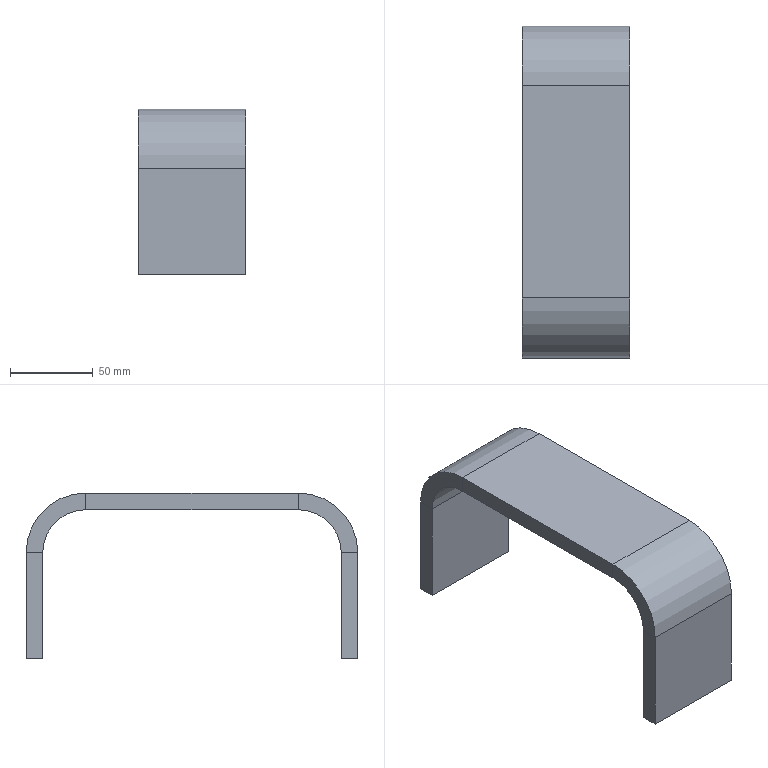Part | SolidWorks | features FlatPattern 1, SM3dBend 1, SMBaseFlange 1, SheetMetal 1 | 1 solid | 22 faces | box 65 x 200.003 x 99.994 mm | volume 229697 mm3 | plane 18 | cylinder 4 | commonest cylinder face diameters 52 x2 72 x2
STEP:
#1=CARTESIAN_POINT('',(904.458,674.984,0.));
#2=VERTEX_POINT('',#1);
#3=CARTESIAN_POINT('',(904.458,802.987,0.));
#4=VERTEX_POINT('',#3);
#5=CARTESIAN_POINT('',(904.458,562.296,0.));
#6=DIRECTION('',(0.,1.,0.));
#7=VECTOR('',#6,1000.);
#8=LINE('',#5,#7);
#9=EDGE_CURVE('',#2,#4,#8,.T.);
#10=ORIENTED_EDGE('',*,*,#9,.T.);
#11=CARTESIAN_POINT('',(839.458,802.987,0.));
#12=VERTEX_POINT('',#11);
#13=CARTESIAN_POINT('',(0.,802.987,0.));
#14=DIRECTION('',(-1.,0.,0.));
#15=VECTOR('',#14,1000.);
#16=LINE('',#13,#15);
#17=EDGE_CURVE('',#4,#12,#16,.T.);
#18=ORIENTED_EDGE('',*,*,#17,.T.);
#19=CARTESIAN_POINT('',(839.458,674.984,0.));
#20=VERTEX_POINT('',#19);
#21=CARTESIAN_POINT('',(839.458,915.676,0.));
#22=DIRECTION('',(0.,-1.,0.));
#23=VECTOR('',#22,1000.);
#24=LINE('',#21,#23);
#25=EDGE_CURVE('',#12,#20,#24,.T.);
#26=ORIENTED_EDGE('',*,*,#25,.T.);
#27=CARTESIAN_POINT('',(0.,674.984,0.));
#28=DIRECTION('',(-1.,0.,0.));
#29=VECTOR('',#28,1000.);
#30=LINE('',#27,#29);
#31=EDGE_CURVE('',#2,#20,#30,.T.);
#32=ORIENTED_EDGE('',*,*,#31,.F.);
#33=EDGE_LOOP('',(#10,#18,#26,#32));
#34=FACE_OUTER_BOUND('',#33,.T.);
#35=CARTESIAN_POINT('',(0.,0.,0.));
#36=DIRECTION('',(0.,0.,-1.));
#37=DIRECTION('',(-1.,0.,0.));
#38=AXIS2_PLACEMENT_3D('',#35,#36,#37);
#39=PLANE('',#38);
#40=ADVANCED_FACE('',(#34),#39,.F.);
#41=CARTESIAN_POINT('',(904.458,802.987,-10.));
#42=VERTEX_POINT('',#41);
#43=CARTESIAN_POINT('',(904.458,802.987,-10.));
#44=DIRECTION('',(0.,0.,-1.));
#45=VECTOR('',#44,1000.);
#46=LINE('',#43,#45);
#47=EDGE_CURVE('',#4,#42,#46,.T.);
#48=ORIENTED_EDGE('',*,*,#47,.F.);
#49=ORIENTED_EDGE('',*,*,#9,.F.);
#50=CARTESIAN_POINT('',(904.458,674.984,-10.));
#51=VERTEX_POINT('',#50);
#52=CARTESIAN_POINT('',(904.458,674.984,-10.));
#53=DIRECTION('',(0.,0.,-1.));
#54=VECTOR('',#53,1000.);
#55=LINE('',#52,#54);
#56=EDGE_CURVE('',#2,#51,#55,.T.);
#57=ORIENTED_EDGE('',*,*,#56,.T.);
#58=CARTESIAN_POINT('',(904.458,562.296,-10.));
#59=DIRECTION('',(0.,1.,0.));
#60=VECTOR('',#59,1000.);
#61=LINE('',#58,#60);
#62=EDGE_CURVE('',#51,#42,#61,.T.);
#63=ORIENTED_EDGE('',*,*,#62,.T.);
#64=EDGE_LOOP('',(#48,#49,#57,#63));
#65=FACE_OUTER_BOUND('',#64,.T.);
#66=CARTESIAN_POINT('',(904.458,562.296,-10.));
#67=DIRECTION('',(1.,0.,0.));
#68=DIRECTION('',(0.,0.,-1.));
#69=AXIS2_PLACEMENT_3D('',#66,#67,#68);
#70=PLANE('',#69);
#71=ADVANCED_FACE('',(#65),#70,.T.);
#72=CARTESIAN_POINT('',(839.458,802.987,-10.));
#73=VERTEX_POINT('',#72);
#74=CARTESIAN_POINT('',(839.458,802.987,-10.));
#75=DIRECTION('',(0.,0.,1.));
#76=VECTOR('',#75,1000.);
#77=LINE('',#74,#76);
#78=EDGE_CURVE('',#73,#12,#77,.T.);
#79=ORIENTED_EDGE('',*,*,#78,.F.);
#80=CARTESIAN_POINT('',(839.458,674.984,-10.));
#81=VERTEX_POINT('',#80);
#82=CARTESIAN_POINT('',(839.458,915.676,-10.));
#83=DIRECTION('',(0.,-1.,0.));
#84=VECTOR('',#83,1000.);
#85=LINE('',#82,#84);
#86=EDGE_CURVE('',#73,#81,#85,.T.);
#87=ORIENTED_EDGE('',*,*,#86,.T.);
#88=CARTESIAN_POINT('',(839.458,674.984,-10.));
#89=DIRECTION('',(0.,0.,1.));
#90=VECTOR('',#89,1000.);
#91=LINE('',#88,#90);
#92=EDGE_CURVE('',#81,#20,#91,.T.);
#93=ORIENTED_EDGE('',*,*,#92,.T.);
#94=ORIENTED_EDGE('',*,*,#25,.F.);
#95=EDGE_LOOP('',(#79,#87,#93,#94));
#96=FACE_OUTER_BOUND('',#95,.T.);
#97=CARTESIAN_POINT('',(839.458,915.676,-10.));
#98=DIRECTION('',(-1.,0.,0.));
#99=DIRECTION('',(0.,0.,1.));
#100=AXIS2_PLACEMENT_3D('',#97,#98,#99);
#101=PLANE('',#100);
#102=ADVANCED_FACE('',(#96),#101,.T.);
#103=CARTESIAN_POINT('',(0.,802.987,-10.));
#104=DIRECTION('',(-1.,0.,0.));
#105=VECTOR('',#104,1000.);
#106=LINE('',#103,#105);
#107=EDGE_CURVE('',#42,#73,#106,.T.);
#108=ORIENTED_EDGE('',*,*,#107,.F.);
#109=ORIENTED_EDGE('',*,*,#62,.F.);
#110=CARTESIAN_POINT('',(0.,674.984,-10.));
#111=DIRECTION('',(-1.,0.,0.));
#112=VECTOR('',#111,1000.);
#113=LINE('',#110,#112);
#114=EDGE_CURVE('',#51,#81,#113,.T.);
#115=ORIENTED_EDGE('',*,*,#114,.T.);
#116=ORIENTED_EDGE('',*,*,#86,.F.);
#117=EDGE_LOOP('',(#108,#109,#115,#116));
#118=FACE_OUTER_BOUND('',#117,.T.);
#119=CARTESIAN_POINT('',(0.,0.,-10.));
#120=DIRECTION('',(0.,0.,-1.));
#121=DIRECTION('',(-1.,0.,0.));
#122=AXIS2_PLACEMENT_3D('',#119,#120,#121);
#123=PLANE('',#122);
#124=ADVANCED_FACE('',(#118),#123,.T.);
#125=ORIENTED_EDGE('',*,*,#56,.F.);
#126=CARTESIAN_POINT('',(904.458,638.984,-36.));
#127=VERTEX_POINT('',#126);
#128=CARTESIAN_POINT('',(904.458,674.984,-36.));
#129=DIRECTION('',(1.,0.,0.));
#130=DIRECTION('',(0.,0.,1.));
#131=AXIS2_PLACEMENT_3D('',#128,#129,#130);
#132=CIRCLE('',#131,36.);
#133=EDGE_CURVE('',#2,#127,#132,.T.);
#134=ORIENTED_EDGE('',*,*,#133,.T.);
#135=CARTESIAN_POINT('',(904.458,648.984,-36.));
#136=VERTEX_POINT('',#135);
#137=CARTESIAN_POINT('',(904.458,648.984,-36.));
#138=DIRECTION('',(0.,1.,0.));
#139=VECTOR('',#138,1000.);
#140=LINE('',#137,#139);
#141=EDGE_CURVE('',#127,#136,#140,.T.);
#142=ORIENTED_EDGE('',*,*,#141,.T.);
#143=CARTESIAN_POINT('',(904.458,674.984,-36.));
#144=DIRECTION('',(1.,0.,0.));
#145=DIRECTION('',(0.,0.,1.));
#146=AXIS2_PLACEMENT_3D('',#143,#144,#145);
#147=CIRCLE('',#146,26.);
#148=EDGE_CURVE('',#51,#136,#147,.T.);
#149=ORIENTED_EDGE('',*,*,#148,.F.);
#150=EDGE_LOOP('',(#125,#134,#142,#149));
#151=FACE_OUTER_BOUND('',#150,.T.);
#152=CARTESIAN_POINT('',(904.458,674.984,-36.));
#153=DIRECTION('',(-1.,0.,0.));
#154=DIRECTION('',(0.,0.,1.));
#155=AXIS2_PLACEMENT_3D('',#152,#153,#154);
#156=PLANE('',#155);
#157=ADVANCED_FACE('',(#151),#156,.F.);
#158=CARTESIAN_POINT('',(839.458,638.984,-36.));
#159=VERTEX_POINT('',#158);
#160=CARTESIAN_POINT('',(839.458,674.984,-36.));
#161=DIRECTION('',(-1.,0.,0.));
#162=DIRECTION('',(0.,0.,1.));
#163=AXIS2_PLACEMENT_3D('',#160,#161,#162);
#164=CIRCLE('',#163,36.);
#165=EDGE_CURVE('',#159,#20,#164,.T.);
#166=ORIENTED_EDGE('',*,*,#165,.T.);
#167=ORIENTED_EDGE('',*,*,#92,.F.);
#168=CARTESIAN_POINT('',(839.458,648.984,-36.));
#169=VERTEX_POINT('',#168);
#170=CARTESIAN_POINT('',(839.458,674.984,-36.));
#171=DIRECTION('',(-1.,0.,0.));
#172=DIRECTION('',(0.,0.,-1.));
#173=AXIS2_PLACEMENT_3D('',#170,#171,#172);
#174=CIRCLE('',#173,26.);
#175=EDGE_CURVE('',#169,#81,#174,.T.);
#176=ORIENTED_EDGE('',*,*,#175,.F.);
#177=CARTESIAN_POINT('',(839.458,648.984,-36.));
#178=DIRECTION('',(0.,-1.,0.));
#179=VECTOR('',#178,1000.);
#180=LINE('',#177,#179);
#181=EDGE_CURVE('',#169,#159,#180,.T.);
#182=ORIENTED_EDGE('',*,*,#181,.T.);
#183=EDGE_LOOP('',(#166,#167,#176,#182));
#184=FACE_OUTER_BOUND('',#183,.T.);
#185=CARTESIAN_POINT('',(839.458,674.984,-36.));
#186=DIRECTION('',(1.,0.,0.));
#187=DIRECTION('',(0.,0.,-1.));
#188=AXIS2_PLACEMENT_3D('',#185,#186,#187);
#189=PLANE('',#188);
#190=ADVANCED_FACE('',(#184),#189,.F.);
#191=CARTESIAN_POINT('',(0.,648.984,-36.));
#192=DIRECTION('',(-1.,0.,0.));
#193=VECTOR('',#192,1000.);
#194=LINE('',#191,#193);
#195=EDGE_CURVE('',#136,#169,#194,.T.);
#196=ORIENTED_EDGE('',*,*,#195,.T.);
#197=ORIENTED_EDGE('',*,*,#175,.T.);
#198=ORIENTED_EDGE('',*,*,#114,.F.);
#199=ORIENTED_EDGE('',*,*,#148,.T.);
#200=EDGE_LOOP('',(#196,#197,#198,#199));
#201=FACE_OUTER_BOUND('',#200,.T.);
#202=CARTESIAN_POINT('',(953.788,674.984,-36.));
#203=DIRECTION('',(-1.,0.,0.));
#204=DIRECTION('',(0.,0.,1.));
#205=AXIS2_PLACEMENT_3D('',#202,#203,#204);
#206=CYLINDRICAL_SURFACE('',#205,26.);
#207=ADVANCED_FACE('',(#201),#206,.F.);
#208=CARTESIAN_POINT('',(0.,638.984,-36.));
#209=DIRECTION('',(-1.,0.,0.));
#210=VECTOR('',#209,1000.);
#211=LINE('',#208,#210);
#212=EDGE_CURVE('',#127,#159,#211,.T.);
#213=ORIENTED_EDGE('',*,*,#212,.F.);
#214=ORIENTED_EDGE('',*,*,#133,.F.);
#215=ORIENTED_EDGE('',*,*,#31,.T.);
#216=ORIENTED_EDGE('',*,*,#165,.F.);
#217=EDGE_LOOP('',(#213,#214,#215,#216));
#218=FACE_OUTER_BOUND('',#217,.T.);
#219=CARTESIAN_POINT('',(953.788,674.984,-36.));
#220=DIRECTION('',(-1.,0.,0.));
#221=DIRECTION('',(0.,0.,1.));
#222=AXIS2_PLACEMENT_3D('',#219,#220,#221);
#223=CYLINDRICAL_SURFACE('',#222,36.);
#224=ADVANCED_FACE('',(#218),#223,.T.);
#225=CARTESIAN_POINT('',(839.458,638.984,-99.994));
#226=VERTEX_POINT('',#225);
#227=CARTESIAN_POINT('',(904.458,638.984,-99.994));
#228=VERTEX_POINT('',#227);
#229=CARTESIAN_POINT('',(839.458,638.984,-99.994));
#230=DIRECTION('',(1.,0.,0.));
#231=VECTOR('',#230,1000.);
#232=LINE('',#229,#231);
#233=EDGE_CURVE('',#226,#228,#232,.T.);
#234=ORIENTED_EDGE('',*,*,#233,.F.);
#235=CARTESIAN_POINT('',(839.458,648.984,-99.994));
#236=VERTEX_POINT('',#235);
#237=CARTESIAN_POINT('',(839.458,648.984,-99.994));
#238=DIRECTION('',(0.,-1.,0.));
#239=VECTOR('',#238,1000.);
#240=LINE('',#237,#239);
#241=EDGE_CURVE('',#236,#226,#240,.T.);
#242=ORIENTED_EDGE('',*,*,#241,.F.);
#243=CARTESIAN_POINT('',(904.458,648.984,-99.994));
#244=VERTEX_POINT('',#243);
#245=CARTESIAN_POINT('',(839.458,648.984,-99.994));
#246=DIRECTION('',(1.,0.,0.));
#247=VECTOR('',#246,1000.);
#248=LINE('',#245,#247);
#249=EDGE_CURVE('',#236,#244,#248,.T.);
#250=ORIENTED_EDGE('',*,*,#249,.T.);
#251=CARTESIAN_POINT('',(904.458,648.984,-99.994));
#252=DIRECTION('',(0.,-1.,0.));
#253=VECTOR('',#252,1000.);
#254=LINE('',#251,#253);
#255=EDGE_CURVE('',#244,#228,#254,.T.);
#256=ORIENTED_EDGE('',*,*,#255,.T.);
#257=EDGE_LOOP('',(#234,#242,#250,#256));
#258=FACE_OUTER_BOUND('',#257,.T.);
#259=CARTESIAN_POINT('',(839.458,648.984,-99.994));
#260=DIRECTION('',(0.,0.,-1.));
#261=DIRECTION('',(1.,0.,0.));
#262=AXIS2_PLACEMENT_3D('',#259,#260,#261);
#263=PLANE('',#262);
#264=ADVANCED_FACE('',(#258),#263,.T.);
#265=ORIENTED_EDGE('',*,*,#195,.F.);
#266=CARTESIAN_POINT('',(904.458,648.984,-99.994));
#267=DIRECTION('',(0.,0.,1.));
#268=VECTOR('',#267,1000.);
#269=LINE('',#266,#268);
#270=EDGE_CURVE('',#244,#136,#269,.T.);
#271=ORIENTED_EDGE('',*,*,#270,.F.);
#272=ORIENTED_EDGE('',*,*,#249,.F.);
#273=CARTESIAN_POINT('',(839.458,648.984,253.386));
#274=DIRECTION('',(0.,0.,-1.));
#275=VECTOR('',#274,1000.);
#276=LINE('',#273,#275);
#277=EDGE_CURVE('',#169,#236,#276,.T.);
#278=ORIENTED_EDGE('',*,*,#277,.F.);
#279=EDGE_LOOP('',(#265,#271,#272,#278));
#280=FACE_OUTER_BOUND('',#279,.T.);
#281=CARTESIAN_POINT('',(0.,648.984,-662.289));
#282=DIRECTION('',(0.,1.,0.));
#283=DIRECTION('',(-1.,0.,0.));
#284=AXIS2_PLACEMENT_3D('',#281,#282,#283);
#285=PLANE('',#284);
#286=ADVANCED_FACE('',(#280),#285,.T.);
#287=ORIENTED_EDGE('',*,*,#141,.F.);
#288=CARTESIAN_POINT('',(904.458,638.984,-99.994));
#289=DIRECTION('',(0.,0.,1.));
#290=VECTOR('',#289,1000.);
#291=LINE('',#288,#290);
#292=EDGE_CURVE('',#228,#127,#291,.T.);
#293=ORIENTED_EDGE('',*,*,#292,.F.);
#294=ORIENTED_EDGE('',*,*,#255,.F.);
#295=ORIENTED_EDGE('',*,*,#270,.T.);
#296=EDGE_LOOP('',(#287,#293,#294,#295));
#297=FACE_OUTER_BOUND('',#296,.T.);
#298=CARTESIAN_POINT('',(904.458,648.984,-99.994));
#299=DIRECTION('',(1.,0.,0.));
#300=DIRECTION('',(0.,1.,0.));
#301=AXIS2_PLACEMENT_3D('',#298,#299,#300);
#302=PLANE('',#301);
#303=ADVANCED_FACE('',(#297),#302,.T.);
#304=ORIENTED_EDGE('',*,*,#292,.T.);
#305=ORIENTED_EDGE('',*,*,#212,.T.);
#306=CARTESIAN_POINT('',(839.458,638.984,253.386));
#307=DIRECTION('',(0.,0.,-1.));
#308=VECTOR('',#307,1000.);
#309=LINE('',#306,#308);
#310=EDGE_CURVE('',#159,#226,#309,.T.);
#311=ORIENTED_EDGE('',*,*,#310,.T.);
#312=ORIENTED_EDGE('',*,*,#233,.T.);
#313=EDGE_LOOP('',(#304,#305,#311,#312));
#314=FACE_OUTER_BOUND('',#313,.T.);
#315=CARTESIAN_POINT('',(0.,638.984,-662.289));
#316=DIRECTION('',(0.,1.,0.));
#317=DIRECTION('',(-1.,0.,0.));
#318=AXIS2_PLACEMENT_3D('',#315,#316,#317);
#319=PLANE('',#318);
#320=ADVANCED_FACE('',(#314),#319,.F.);
#321=ORIENTED_EDGE('',*,*,#181,.F.);
#322=ORIENTED_EDGE('',*,*,#277,.T.);
#323=ORIENTED_EDGE('',*,*,#241,.T.);
#324=ORIENTED_EDGE('',*,*,#310,.F.);
#325=EDGE_LOOP('',(#321,#322,#323,#324));
#326=FACE_OUTER_BOUND('',#325,.T.);
#327=CARTESIAN_POINT('',(839.458,648.984,253.386));
#328=DIRECTION('',(-1.,0.,0.));
#329=DIRECTION('',(0.,-1.,0.));
#330=AXIS2_PLACEMENT_3D('',#327,#328,#329);
#331=PLANE('',#330);
#332=ADVANCED_FACE('',(#326),#331,.T.);
#333=CARTESIAN_POINT('',(904.458,838.987,-36.));
#334=VERTEX_POINT('',#333);
#335=CARTESIAN_POINT('',(904.458,828.987,-36.));
#336=VERTEX_POINT('',#335);
#337=CARTESIAN_POINT('',(904.458,828.987,-36.));
#338=DIRECTION('',(0.,-1.,0.));
#339=VECTOR('',#338,1000.);
#340=LINE('',#337,#339);
#341=EDGE_CURVE('',#334,#336,#340,.T.);
#342=ORIENTED_EDGE('',*,*,#341,.F.);
#343=CARTESIAN_POINT('',(904.458,802.987,-36.));
#344=DIRECTION('',(1.,0.,0.));
#345=DIRECTION('',(0.,0.,-1.));
#346=AXIS2_PLACEMENT_3D('',#343,#344,#345);
#347=CIRCLE('',#346,36.);
#348=EDGE_CURVE('',#334,#4,#347,.T.);
#349=ORIENTED_EDGE('',*,*,#348,.T.);
#350=ORIENTED_EDGE('',*,*,#47,.T.);
#351=CARTESIAN_POINT('',(904.458,802.987,-36.));
#352=DIRECTION('',(1.,0.,0.));
#353=DIRECTION('',(0.,0.,1.));
#354=AXIS2_PLACEMENT_3D('',#351,#352,#353);
#355=CIRCLE('',#354,26.);
#356=EDGE_CURVE('',#336,#42,#355,.T.);
#357=ORIENTED_EDGE('',*,*,#356,.F.);
#358=EDGE_LOOP('',(#342,#349,#350,#357));
#359=FACE_OUTER_BOUND('',#358,.T.);
#360=CARTESIAN_POINT('',(904.458,802.987,-36.));
#361=DIRECTION('',(-1.,0.,0.));
#362=DIRECTION('',(0.,0.,1.));
#363=AXIS2_PLACEMENT_3D('',#360,#361,#362);
#364=PLANE('',#363);
#365=ADVANCED_FACE('',(#359),#364,.F.);
#366=CARTESIAN_POINT('',(839.458,838.987,-36.));
#367=VERTEX_POINT('',#366);
#368=CARTESIAN_POINT('',(839.458,802.987,-36.));
#369=DIRECTION('',(-1.,0.,0.));
#370=DIRECTION('',(0.,0.,-1.));
#371=AXIS2_PLACEMENT_3D('',#368,#369,#370);
#372=CIRCLE('',#371,36.);
#373=EDGE_CURVE('',#12,#367,#372,.T.);
#374=ORIENTED_EDGE('',*,*,#373,.T.);
#375=CARTESIAN_POINT('',(839.458,828.987,-36.));
#376=VERTEX_POINT('',#375);
#377=CARTESIAN_POINT('',(839.458,828.987,-36.));
#378=DIRECTION('',(0.,1.,0.));
#379=VECTOR('',#378,1000.);
#380=LINE('',#377,#379);
#381=EDGE_CURVE('',#376,#367,#380,.T.);
#382=ORIENTED_EDGE('',*,*,#381,.F.);
#383=CARTESIAN_POINT('',(839.458,802.987,-36.));
#384=DIRECTION('',(-1.,0.,0.));
#385=DIRECTION('',(0.,0.,-1.));
#386=AXIS2_PLACEMENT_3D('',#383,#384,#385);
#387=CIRCLE('',#386,26.);
#388=EDGE_CURVE('',#73,#376,#387,.T.);
#389=ORIENTED_EDGE('',*,*,#388,.F.);
#390=ORIENTED_EDGE('',*,*,#78,.T.);
#391=EDGE_LOOP('',(#374,#382,#389,#390));
#392=FACE_OUTER_BOUND('',#391,.T.);
#393=CARTESIAN_POINT('',(839.458,802.987,-36.));
#394=DIRECTION('',(1.,0.,0.));
#395=DIRECTION('',(0.,0.,-1.));
#396=AXIS2_PLACEMENT_3D('',#393,#394,#395);
#397=PLANE('',#396);
#398=ADVANCED_FACE('',(#392),#397,.F.);
#399=ORIENTED_EDGE('',*,*,#107,.T.);
#400=ORIENTED_EDGE('',*,*,#388,.T.);
#401=CARTESIAN_POINT('',(0.,828.987,-36.));
#402=DIRECTION('',(-1.,0.,0.));
#403=VECTOR('',#402,1000.);
#404=LINE('',#401,#403);
#405=EDGE_CURVE('',#336,#376,#404,.T.);
#406=ORIENTED_EDGE('',*,*,#405,.F.);
#407=ORIENTED_EDGE('',*,*,#356,.T.);
#408=EDGE_LOOP('',(#399,#400,#406,#407));
#409=FACE_OUTER_BOUND('',#408,.T.);
#410=CARTESIAN_POINT('',(790.128,802.987,-36.));
#411=DIRECTION('',(1.,0.,0.));
#412=DIRECTION('',(0.,0.,-1.));
#413=AXIS2_PLACEMENT_3D('',#410,#411,#412);
#414=CYLINDRICAL_SURFACE('',#413,26.);
#415=ADVANCED_FACE('',(#409),#414,.F.);
#416=ORIENTED_EDGE('',*,*,#17,.F.);
#417=ORIENTED_EDGE('',*,*,#348,.F.);
#418=CARTESIAN_POINT('',(0.,838.987,-36.));
#419=DIRECTION('',(-1.,0.,0.));
#420=VECTOR('',#419,1000.);
#421=LINE('',#418,#420);
#422=EDGE_CURVE('',#334,#367,#421,.T.);
#423=ORIENTED_EDGE('',*,*,#422,.T.);
#424=ORIENTED_EDGE('',*,*,#373,.F.);
#425=EDGE_LOOP('',(#416,#417,#423,#424));
#426=FACE_OUTER_BOUND('',#425,.T.);
#427=CARTESIAN_POINT('',(790.128,802.987,-36.));
#428=DIRECTION('',(1.,0.,0.));
#429=DIRECTION('',(0.,0.,-1.));
#430=AXIS2_PLACEMENT_3D('',#427,#428,#429);
#431=CYLINDRICAL_SURFACE('',#430,36.);
#432=ADVANCED_FACE('',(#426),#431,.T.);
#433=CARTESIAN_POINT('',(904.458,838.987,-99.994));
#434=VERTEX_POINT('',#433);
#435=CARTESIAN_POINT('',(839.458,838.987,-99.994));
#436=VERTEX_POINT('',#435);
#437=CARTESIAN_POINT('',(839.458,838.987,-99.994));
#438=DIRECTION('',(-1.,0.,0.));
#439=VECTOR('',#438,1000.);
#440=LINE('',#437,#439);
#441=EDGE_CURVE('',#434,#436,#440,.T.);
#442=ORIENTED_EDGE('',*,*,#441,.F.);
#443=CARTESIAN_POINT('',(904.458,828.987,-99.994));
#444=VERTEX_POINT('',#443);
#445=CARTESIAN_POINT('',(904.458,828.987,-99.994));
#446=DIRECTION('',(0.,1.,0.));
#447=VECTOR('',#446,1000.);
#448=LINE('',#445,#447);
#449=EDGE_CURVE('',#444,#434,#448,.T.);
#450=ORIENTED_EDGE('',*,*,#449,.F.);
#451=CARTESIAN_POINT('',(839.458,828.987,-99.994));
#452=VERTEX_POINT('',#451);
#453=CARTESIAN_POINT('',(839.458,828.987,-99.994));
#454=DIRECTION('',(-1.,0.,0.));
#455=VECTOR('',#454,1000.);
#456=LINE('',#453,#455);
#457=EDGE_CURVE('',#444,#452,#456,.T.);
#458=ORIENTED_EDGE('',*,*,#457,.T.);
#459=CARTESIAN_POINT('',(839.458,828.987,-99.994));
#460=DIRECTION('',(0.,1.,0.));
#461=VECTOR('',#460,1000.);
#462=LINE('',#459,#461);
#463=EDGE_CURVE('',#452,#436,#462,.T.);
#464=ORIENTED_EDGE('',*,*,#463,.T.);
#465=EDGE_LOOP('',(#442,#450,#458,#464));
#466=FACE_OUTER_BOUND('',#465,.T.);
#467=CARTESIAN_POINT('',(839.458,828.987,-99.994));
#468=DIRECTION('',(0.,0.,-1.));
#469=DIRECTION('',(0.,1.,0.));
#470=AXIS2_PLACEMENT_3D('',#467,#468,#469);
#471=PLANE('',#470);
#472=ADVANCED_FACE('',(#466),#471,.T.);
#473=CARTESIAN_POINT('',(904.458,828.987,253.386));
#474=DIRECTION('',(0.,0.,-1.));
#475=VECTOR('',#474,1000.);
#476=LINE('',#473,#475);
#477=EDGE_CURVE('',#336,#444,#476,.T.);
#478=ORIENTED_EDGE('',*,*,#477,.F.);
#479=ORIENTED_EDGE('',*,*,#405,.T.);
#480=CARTESIAN_POINT('',(839.458,828.987,-99.994));
#481=DIRECTION('',(0.,0.,1.));
#482=VECTOR('',#481,1000.);
#483=LINE('',#480,#482);
#484=EDGE_CURVE('',#452,#376,#483,.T.);
#485=ORIENTED_EDGE('',*,*,#484,.F.);
#486=ORIENTED_EDGE('',*,*,#457,.F.);
#487=EDGE_LOOP('',(#478,#479,#485,#486));
#488=FACE_OUTER_BOUND('',#487,.T.);
#489=CARTESIAN_POINT('',(0.,828.987,815.682));
#490=DIRECTION('',(0.,-1.,0.));
#491=DIRECTION('',(-1.,0.,0.));
#492=AXIS2_PLACEMENT_3D('',#489,#490,#491);
#493=PLANE('',#492);
#494=ADVANCED_FACE('',(#488),#493,.T.);
#495=ORIENTED_EDGE('',*,*,#484,.T.);
#496=ORIENTED_EDGE('',*,*,#381,.T.);
#497=CARTESIAN_POINT('',(839.458,838.987,-99.994));
#498=DIRECTION('',(0.,0.,1.));
#499=VECTOR('',#498,1000.);
#500=LINE('',#497,#499);
#501=EDGE_CURVE('',#436,#367,#500,.T.);
#502=ORIENTED_EDGE('',*,*,#501,.F.);
#503=ORIENTED_EDGE('',*,*,#463,.F.);
#504=EDGE_LOOP('',(#495,#496,#502,#503));
#505=FACE_OUTER_BOUND('',#504,.T.);
#506=CARTESIAN_POINT('',(839.458,828.987,-99.994));
#507=DIRECTION('',(-1.,0.,0.));
#508=DIRECTION('',(0.,1.,0.));
#509=AXIS2_PLACEMENT_3D('',#506,#507,#508);
#510=PLANE('',#509);
#511=ADVANCED_FACE('',(#505),#510,.T.);
#512=ORIENTED_EDGE('',*,*,#422,.F.);
#513=CARTESIAN_POINT('',(904.458,838.987,253.386));
#514=DIRECTION('',(0.,0.,-1.));
#515=VECTOR('',#514,1000.);
#516=LINE('',#513,#515);
#517=EDGE_CURVE('',#334,#434,#516,.T.);
#518=ORIENTED_EDGE('',*,*,#517,.T.);
#519=ORIENTED_EDGE('',*,*,#441,.T.);
#520=ORIENTED_EDGE('',*,*,#501,.T.);
#521=EDGE_LOOP('',(#512,#518,#519,#520));
#522=FACE_OUTER_BOUND('',#521,.T.);
#523=CARTESIAN_POINT('',(0.,838.987,815.682));
#524=DIRECTION('',(0.,-1.,0.));
#525=DIRECTION('',(-1.,0.,0.));
#526=AXIS2_PLACEMENT_3D('',#523,#524,#525);
#527=PLANE('',#526);
#528=ADVANCED_FACE('',(#522),#527,.F.);
#529=ORIENTED_EDGE('',*,*,#517,.F.);
#530=ORIENTED_EDGE('',*,*,#341,.T.);
#531=ORIENTED_EDGE('',*,*,#477,.T.);
#532=ORIENTED_EDGE('',*,*,#449,.T.);
#533=EDGE_LOOP('',(#529,#530,#531,#532));
#534=FACE_OUTER_BOUND('',#533,.T.);
#535=CARTESIAN_POINT('',(904.458,828.987,253.386));
#536=DIRECTION('',(1.,0.,0.));
#537=DIRECTION('',(0.,-1.,0.));
#538=AXIS2_PLACEMENT_3D('',#535,#536,#537);
#539=PLANE('',#538);
#540=ADVANCED_FACE('',(#534),#539,.T.);
#541=CLOSED_SHELL('',(#40,#71,#102,#124,#157,#190,#207,#224,#264,#286,#303,#320,#332,#365,#398,#415,#432,#472,#494,#511,#528,#540));
#542=MANIFOLD_SOLID_BREP('',#541);
#543=CARTESIAN_POINT('',(0.,0.,0.));
#544=DIRECTION('',(0.,0.,1.));
#545=DIRECTION('',(1.,0.,0.));
#546=AXIS2_PLACEMENT_3D('',#543,#544,#545);
#547=(LENGTH_UNIT()NAMED_UNIT(*)SI_UNIT(.MILLI.,.METRE.));
#548=UNCERTAINTY_MEASURE_WITH_UNIT(LENGTH_MEASURE(0.00001),#547,'','');
#549=(NAMED_UNIT(*)PLANE_ANGLE_UNIT()SI_UNIT($,.RADIAN.));
#550=(NAMED_UNIT(*)SI_UNIT($,.STERADIAN.)SOLID_ANGLE_UNIT());
#551=(GEOMETRIC_REPRESENTATION_CONTEXT(3)GLOBAL_UNCERTAINTY_ASSIGNED_CONTEXT((#548))GLOBAL_UNIT_ASSIGNED_CONTEXT((#547,#549,#550))REPRESENTATION_CONTEXT('',''));
#552=ADVANCED_BREP_SHAPE_REPRESENTATION('',(#542,#546),#551);